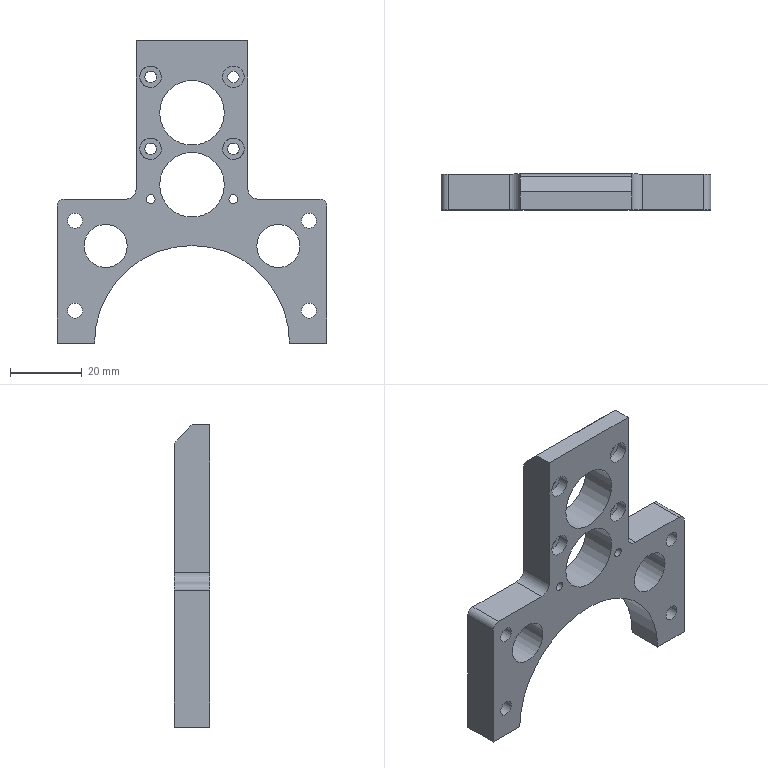CAM job | NX | 3+2 milling, drilling | part box 75 x 10 x 84 mm | stock box 80 x 12 x 89 mm
Tools:
number,name,description,diameter,corner_radius,flute_length,length,flutes
4,D4,平底铣刀-粗,4.0,0.0,25.0,75.0,2
6,D6,平底铣刀-粗,6.0,0.0,25.0,75.0,2
9,D10,平底铣刀-粗,10.0,0.0,35.0,75.0,2
11,D4-J,平底铣刀-精,4.0,0.0,50.0,75.0,2
7,D6-J,平底铣刀-精,6.0,0.0,25.0,75.0,2
10,D10-J,平底铣刀-精,10.0,0.0,35.0,75.0,2
2,D6倒角刀,倒角刀,6.0,0.0,3.0,25.0,2
14,ZT4.2,钻头,4.2,0.0,35.0,50.0,2
18,ZT10,钻头,10.0,0.0,35.0,50.0,2
12,钻头2.5,Twist Drill 2.5 mm,2.5,0.0,30.0,32.0,2
17,ZT3.2,Drilling Tool,3.2,0.0,35.0,50.0,2
Operations:
program,operation,operation_type,tool,method,geometry_group,spindle_rpm,surface_speed,feed_per_tooth,feed_cut,feed_plunge,cut_length_mm,path_length_mm,cut_time_min,machine_time_min
B,DYNAMICROUGHD10_COPY_1,CavityMilling,D10,DYNAMICROUGH-DEPTHK-STEPK,W-B,8000.0,251.32,0.25,4000.0,100.0,15684.378,15780.178,3.921,3.931
B,DRILLCHAMFER_2,Operation,D6倒角刀,METHOD,W-B,8000.0,150.796,0.0625,1000.0,0.0,9.5,145.195,0.0095,0.0231
B,DRILLCHAMFER_3,Operation,D6倒角刀,METHOD,W-B,8000.0,150.796,0.0625,1000.0,0.0,19.6,211.842,0.0196,0.0388
B,DRILLCHAMFER_4,Operation,D6倒角刀,METHOD,W-B,8000.0,150.796,0.0625,1000.0,0.0,22.8,270.028,0.0228,0.0475
B,MILLCHAMFER_4,PlanarMilling,D6倒角刀,METHOD,W-B,8000.0,150.796,0.075,1200.0,100.0,87.451,343.451,0.0729,0.0985
B,PLANARDEBURR6X45L_COPY,SurfaceContour,D6倒角刀,WALLCHAMFER-DEPTH0-STEPG,W-B,6500.0,122.519,0.1154,1500.0,100.0,561.276,1124.382,0.3742,0.4305
B,ZLEVELZIGZAGWALL_COPY,ZLevelMilling,D6-J,ZLEVELWALL-DEPTHK-STEPG,W-B,8000.0,150.796,0.1875,3000.0,100.0,17405.443,17433.551,5.802,5.805
B,TOPFACE_COPY,FaceMilling,D10-J,SIDEFINISH-DEPTHK-STEPG,W-B,4500.0,1385.0,0.1667,1500.0,100.0,1213.923,1309.923,0.8093,0.8189
A,C0.3CLOSEDCONTOURCHAMFER6X45L_COPY,PlanarMilling,D6倒角刀,WALLCHAMFER-DEPTH0-STEPG,W-A,7000.0,131.0,0.1071,1500.0,100.0,361.507,457.507,0.241,0.2506
A,C0.3CLOSEDCONTOURCHAMFER6X45L_COPY_1,PlanarMilling,D6倒角刀,WALLCHAMFER-DEPTH0-STEPG,W-A,7000.0,131.0,0.1071,1500.0,100.0,223.836,696.862,0.1492,0.1965
A,DYNAMICROUGHD10_COPY,CavityMilling,D10,DYNAMICROUGH-DEPTHK-STEPK,W-A,8000.0,251.32,0.25,4000.0,100.0,9030.922,9146.922,2.258,2.269
A,TOPFACE,FaceMilling,D10-J,SIDEFINISH-DEPTHK-STEPG,W-A,4500.0,1385.0,0.1667,1500.0,100.0,1213.923,1309.923,0.8093,0.8189
A,SPOT,Operation,D6倒角刀,METHOD,W-A,3000.0,56.549,0.0333,200.0,0.0,4.0,132.022,0.02,0.0328
A,SPOT_2,Operation,D6倒角刀,METHOD,W-A,3000.0,56.549,0.0333,200.0,0.0,30.0,381.879,0.15,0.1852
A,HOLEDRILL,Operation,钻头2.5,METHOD,W-A,3800.0,29.845,0.0105,80.0,0.0,26.502,177.026,0.3313,0.3463
A,HOLEDRILL_3,Operation,ZT3.2,METHOD,W-A,3000.0,30.159,0.02,120.0,0.0,51.695,269.462,0.4308,0.4526
A,HOLEDRILL_2,Operation,ZT4.2,METHOD,W-A,3000.0,39.584,0.0167,100.0,0.0,55.047,328.142,0.5505,0.5778
A,HOLEDRILL_4,Operation,ZT10,METHOD,W-A,2000.0,62.832,0.0375,150.0,0.0,30.009,209.028,0.2001,0.218
A,HOLEDRILL_5,Operation,ZT10,METHOD,W-A,2000.0,62.832,0.03,120.0,0.0,31.009,183.042,0.2584,0.2736
A,HOLEROUGH_3,CylinderMilling,D6,METHOD,W-A,6000.0,113.097,0.1667,2000.0,100.0,805.661,1073.061,0.4028,0.4296
A,HOLEROUGHD6_3,CylinderMilling,D6,METHOD,W-A,6000.0,157.0,0.1667,2000.0,90.0,3059.464,3298.464,1.531,1.554
A,HOLEROUGH_1,CylinderMilling,D4,METHOD,W-A,6000.0,75.398,0.1,1200.0,100.0,210.474,435.874,0.1754,0.1979
A,HOLEROUGH_2,CylinderMilling,D4,METHOD,W-A,6000.0,75.398,0.1,1200.0,100.0,210.474,435.874,0.1754,0.1979
A,HOLESIDE_3,CylinderMilling,D6-J,METHOD,W-A,6000.0,113.097,0.0417,500.0,100.0,103.316,391.316,0.2066,0.2354
A,HOLESIDEE6_3,CylinderMilling,D6-J,METHOD,W-A,6000.0,157.0,0.2,800.0,90.0,171.748,435.213,0.216,0.2423
A,HOLESIDE_1,CylinderMilling,D4-J,METHOD,W-A,6000.0,75.398,0.05,600.0,100.0,18.52,250.519,0.0309,0.0541
A,HOLESIDE_2,CylinderMilling,D4-J,METHOD,W-A,6000.0,75.398,0.05,600.0,100.0,18.52,250.519,0.0309,0.0541
A,ZLEVELSMOOTHCORNERD6REF12_COPY,ZLevelMilling,D6-J,LAYERFINISH-DEPTHK-STEPG,W-A,8000.0,150.796,0.125,2000.0,100.0,433.637,690.44,0.2168,0.2425
A,SELECTEDBODYONLY,SurfaceContour,D6倒角刀,METHOD,W-A,8000.0,150.796,0.1875,3000.0,100.0,477.121,816.113,0.159,0.1929
A,DRILLCHAMFER_1,Operation,D6倒角刀,METHOD,W-A,5000.0,94.248,0.015,150.0,0.0,9.5,145.195,0.0633,0.0769
A,MILLCHAMFER_1,PlanarMilling,D6倒角刀,METHOD,W-A,6000.0,113.097,0.05,600.0,100.0,49.927,570.609,0.0832,0.1353
A,MILLCHAMFER_2,PlanarMilling,D6倒角刀,METHOD,W-A,6000.0,113.097,0.05,600.0,100.0,47.132,522.149,0.0786,0.1261
A,MILLCHAMFER_3,PlanarMilling,D6倒角刀,METHOD,W-A,6000.0,113.097,0.05,600.0,100.0,81.168,327.168,0.1353,0.1599
A,CONTOURSEMIFINISH_2,VolumeBased25DMillingOperation,D6-J,METHOD,W-A,9000.0,169.646,0.0667,1200.0,100.0,368.411,487.411,0.307,0.3189